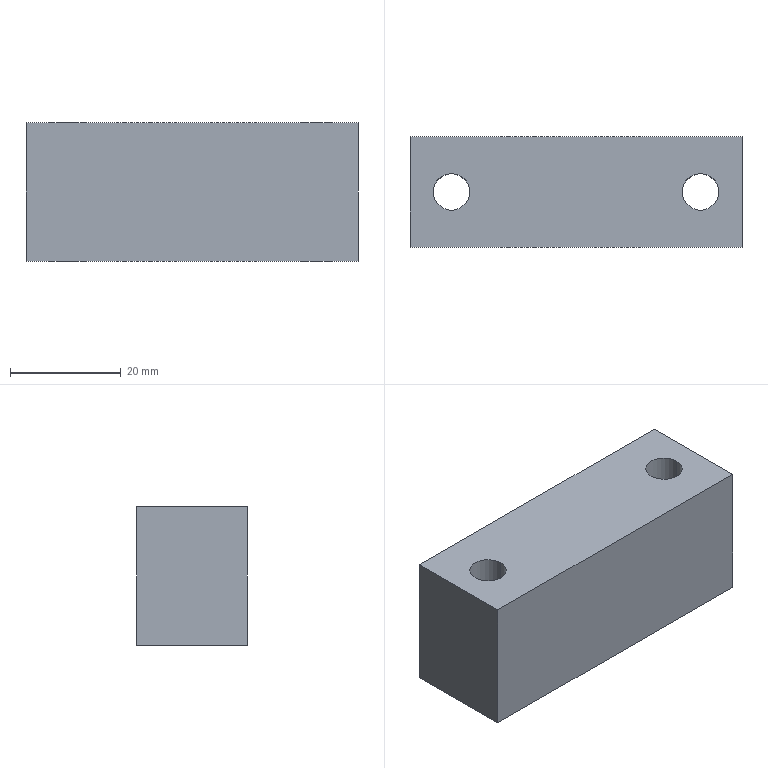Part | SolidWorks | features Extrusion 1, HoleWzd 1 | 1 solid | 10 faces | box 60 x 20 x 25 mm | volume 28289 mm3 | plane 6 | cylinder 4 | commonest cylinder face diameters 6.6 x4
STEP:
#1=CARTESIAN_POINT('',(-25.8,0.,0.));
#2=VERTEX_POINT('',#1);
#3=CARTESIAN_POINT('',(-19.2,0.,0.));
#4=VERTEX_POINT('',#3);
#5=CARTESIAN_POINT('',(-22.5,0.,0.));
#6=DIRECTION('',(0.,0.,1.));
#7=DIRECTION('',(1.,0.,0.));
#8=AXIS2_PLACEMENT_3D('',#5,#6,#7);
#9=CIRCLE('',#8,3.3);
#10=EDGE_CURVE('',#2,#4,#9,.T.);
#11=ORIENTED_EDGE('',*,*,#10,.F.);
#12=CARTESIAN_POINT('',(-25.8,0.,25.));
#13=VERTEX_POINT('',#12);
#14=CARTESIAN_POINT('',(-25.8,0.,25.));
#15=DIRECTION('',(0.,0.,1.));
#16=VECTOR('',#15,1000.);
#17=LINE('',#14,#16);
#18=EDGE_CURVE('',#2,#13,#17,.T.);
#19=ORIENTED_EDGE('',*,*,#18,.T.);
#20=CARTESIAN_POINT('',(-19.2,0.,25.));
#21=VERTEX_POINT('',#20);
#22=CARTESIAN_POINT('',(-22.5,0.,25.));
#23=DIRECTION('',(0.,0.,1.));
#24=DIRECTION('',(1.,0.,0.));
#25=AXIS2_PLACEMENT_3D('',#22,#23,#24);
#26=CIRCLE('',#25,3.3);
#27=EDGE_CURVE('',#13,#21,#26,.T.);
#28=ORIENTED_EDGE('',*,*,#27,.T.);
#29=CARTESIAN_POINT('',(-19.2,0.,25.));
#30=DIRECTION('',(0.,0.,1.));
#31=VECTOR('',#30,1000.);
#32=LINE('',#29,#31);
#33=EDGE_CURVE('',#4,#21,#32,.T.);
#34=ORIENTED_EDGE('',*,*,#33,.F.);
#35=EDGE_LOOP('',(#11,#19,#28,#34));
#36=FACE_OUTER_BOUND('',#35,.T.);
#37=CARTESIAN_POINT('',(-22.5,0.,25.));
#38=DIRECTION('',(0.,0.,1.));
#39=DIRECTION('',(1.,0.,0.));
#40=AXIS2_PLACEMENT_3D('',#37,#38,#39);
#41=CYLINDRICAL_SURFACE('',#40,3.3);
#42=ADVANCED_FACE('',(#36),#41,.F.);
#43=CARTESIAN_POINT('',(19.2,0.,0.));
#44=VERTEX_POINT('',#43);
#45=CARTESIAN_POINT('',(25.8,0.,0.));
#46=VERTEX_POINT('',#45);
#47=CARTESIAN_POINT('',(22.5,0.,0.));
#48=DIRECTION('',(0.,0.,1.));
#49=DIRECTION('',(1.,0.,0.));
#50=AXIS2_PLACEMENT_3D('',#47,#48,#49);
#51=CIRCLE('',#50,3.3);
#52=EDGE_CURVE('',#44,#46,#51,.T.);
#53=ORIENTED_EDGE('',*,*,#52,.F.);
#54=CARTESIAN_POINT('',(19.2,0.,25.));
#55=VERTEX_POINT('',#54);
#56=CARTESIAN_POINT('',(19.2,0.,25.));
#57=DIRECTION('',(0.,0.,1.));
#58=VECTOR('',#57,1000.);
#59=LINE('',#56,#58);
#60=EDGE_CURVE('',#44,#55,#59,.T.);
#61=ORIENTED_EDGE('',*,*,#60,.T.);
#62=CARTESIAN_POINT('',(25.8,0.,25.));
#63=VERTEX_POINT('',#62);
#64=CARTESIAN_POINT('',(22.5,0.,25.));
#65=DIRECTION('',(0.,0.,1.));
#66=DIRECTION('',(1.,0.,0.));
#67=AXIS2_PLACEMENT_3D('',#64,#65,#66);
#68=CIRCLE('',#67,3.3);
#69=EDGE_CURVE('',#55,#63,#68,.T.);
#70=ORIENTED_EDGE('',*,*,#69,.T.);
#71=CARTESIAN_POINT('',(25.8,0.,25.));
#72=DIRECTION('',(0.,0.,1.));
#73=VECTOR('',#72,1000.);
#74=LINE('',#71,#73);
#75=EDGE_CURVE('',#46,#63,#74,.T.);
#76=ORIENTED_EDGE('',*,*,#75,.F.);
#77=EDGE_LOOP('',(#53,#61,#70,#76));
#78=FACE_OUTER_BOUND('',#77,.T.);
#79=CARTESIAN_POINT('',(22.5,0.,25.));
#80=DIRECTION('',(0.,0.,1.));
#81=DIRECTION('',(1.,0.,0.));
#82=AXIS2_PLACEMENT_3D('',#79,#80,#81);
#83=CYLINDRICAL_SURFACE('',#82,3.3);
#84=ADVANCED_FACE('',(#78),#83,.F.);
#85=CARTESIAN_POINT('',(-30.,10.,0.));
#86=VERTEX_POINT('',#85);
#87=CARTESIAN_POINT('',(-30.,-10.,0.));
#88=VERTEX_POINT('',#87);
#89=CARTESIAN_POINT('',(-30.,-10.,0.));
#90=DIRECTION('',(0.,-1.,0.));
#91=VECTOR('',#90,1000.);
#92=LINE('',#89,#91);
#93=EDGE_CURVE('',#86,#88,#92,.T.);
#94=ORIENTED_EDGE('',*,*,#93,.T.);
#95=CARTESIAN_POINT('',(-30.,-10.,25.));
#96=VERTEX_POINT('',#95);
#97=CARTESIAN_POINT('',(-30.,-10.,25.));
#98=DIRECTION('',(0.,0.,-1.));
#99=VECTOR('',#98,1000.);
#100=LINE('',#97,#99);
#101=EDGE_CURVE('',#96,#88,#100,.T.);
#102=ORIENTED_EDGE('',*,*,#101,.F.);
#103=CARTESIAN_POINT('',(-30.,10.,25.));
#104=VERTEX_POINT('',#103);
#105=CARTESIAN_POINT('',(-30.,-10.,25.));
#106=DIRECTION('',(0.,-1.,0.));
#107=VECTOR('',#106,1000.);
#108=LINE('',#105,#107);
#109=EDGE_CURVE('',#104,#96,#108,.T.);
#110=ORIENTED_EDGE('',*,*,#109,.F.);
#111=CARTESIAN_POINT('',(-30.,10.,25.));
#112=DIRECTION('',(0.,0.,-1.));
#113=VECTOR('',#112,1000.);
#114=LINE('',#111,#113);
#115=EDGE_CURVE('',#104,#86,#114,.T.);
#116=ORIENTED_EDGE('',*,*,#115,.T.);
#117=EDGE_LOOP('',(#94,#102,#110,#116));
#118=FACE_OUTER_BOUND('',#117,.T.);
#119=CARTESIAN_POINT('',(-30.,-10.,25.));
#120=DIRECTION('',(1.,0.,0.));
#121=DIRECTION('',(0.,0.,-1.));
#122=AXIS2_PLACEMENT_3D('',#119,#120,#121);
#123=PLANE('',#122);
#124=ADVANCED_FACE('',(#118),#123,.F.);
#125=CARTESIAN_POINT('',(30.,-10.,0.));
#126=VERTEX_POINT('',#125);
#127=CARTESIAN_POINT('',(30.,-10.,0.));
#128=DIRECTION('',(1.,0.,0.));
#129=VECTOR('',#128,1000.);
#130=LINE('',#127,#129);
#131=EDGE_CURVE('',#88,#126,#130,.T.);
#132=ORIENTED_EDGE('',*,*,#131,.T.);
#133=CARTESIAN_POINT('',(30.,-10.,25.));
#134=VERTEX_POINT('',#133);
#135=CARTESIAN_POINT('',(30.,-10.,25.));
#136=DIRECTION('',(0.,0.,-1.));
#137=VECTOR('',#136,1000.);
#138=LINE('',#135,#137);
#139=EDGE_CURVE('',#134,#126,#138,.T.);
#140=ORIENTED_EDGE('',*,*,#139,.F.);
#141=CARTESIAN_POINT('',(30.,-10.,25.));
#142=DIRECTION('',(1.,0.,0.));
#143=VECTOR('',#142,1000.);
#144=LINE('',#141,#143);
#145=EDGE_CURVE('',#96,#134,#144,.T.);
#146=ORIENTED_EDGE('',*,*,#145,.F.);
#147=ORIENTED_EDGE('',*,*,#101,.T.);
#148=EDGE_LOOP('',(#132,#140,#146,#147));
#149=FACE_OUTER_BOUND('',#148,.T.);
#150=CARTESIAN_POINT('',(30.,-10.,25.));
#151=DIRECTION('',(0.,1.,0.));
#152=DIRECTION('',(-1.,0.,0.));
#153=AXIS2_PLACEMENT_3D('',#150,#151,#152);
#154=PLANE('',#153);
#155=ADVANCED_FACE('',(#149),#154,.F.);
#156=CARTESIAN_POINT('',(30.,10.,0.));
#157=VERTEX_POINT('',#156);
#158=CARTESIAN_POINT('',(30.,-10.,0.));
#159=DIRECTION('',(0.,1.,0.));
#160=VECTOR('',#159,1000.);
#161=LINE('',#158,#160);
#162=EDGE_CURVE('',#126,#157,#161,.T.);
#163=ORIENTED_EDGE('',*,*,#162,.T.);
#164=CARTESIAN_POINT('',(30.,10.,25.));
#165=VERTEX_POINT('',#164);
#166=CARTESIAN_POINT('',(30.,10.,25.));
#167=DIRECTION('',(0.,0.,-1.));
#168=VECTOR('',#167,1000.);
#169=LINE('',#166,#168);
#170=EDGE_CURVE('',#165,#157,#169,.T.);
#171=ORIENTED_EDGE('',*,*,#170,.F.);
#172=CARTESIAN_POINT('',(30.,-10.,25.));
#173=DIRECTION('',(0.,1.,0.));
#174=VECTOR('',#173,1000.);
#175=LINE('',#172,#174);
#176=EDGE_CURVE('',#134,#165,#175,.T.);
#177=ORIENTED_EDGE('',*,*,#176,.F.);
#178=ORIENTED_EDGE('',*,*,#139,.T.);
#179=EDGE_LOOP('',(#163,#171,#177,#178));
#180=FACE_OUTER_BOUND('',#179,.T.);
#181=CARTESIAN_POINT('',(30.,-10.,25.));
#182=DIRECTION('',(-1.,0.,0.));
#183=DIRECTION('',(0.,0.,1.));
#184=AXIS2_PLACEMENT_3D('',#181,#182,#183);
#185=PLANE('',#184);
#186=ADVANCED_FACE('',(#180),#185,.F.);
#187=CARTESIAN_POINT('',(30.,10.,0.));
#188=DIRECTION('',(-1.,0.,0.));
#189=VECTOR('',#188,1000.);
#190=LINE('',#187,#189);
#191=EDGE_CURVE('',#157,#86,#190,.T.);
#192=ORIENTED_EDGE('',*,*,#191,.T.);
#193=ORIENTED_EDGE('',*,*,#115,.F.);
#194=CARTESIAN_POINT('',(30.,10.,25.));
#195=DIRECTION('',(-1.,0.,0.));
#196=VECTOR('',#195,1000.);
#197=LINE('',#194,#196);
#198=EDGE_CURVE('',#165,#104,#197,.T.);
#199=ORIENTED_EDGE('',*,*,#198,.F.);
#200=ORIENTED_EDGE('',*,*,#170,.T.);
#201=EDGE_LOOP('',(#192,#193,#199,#200));
#202=FACE_OUTER_BOUND('',#201,.T.);
#203=CARTESIAN_POINT('',(30.,10.,25.));
#204=DIRECTION('',(0.,-1.,0.));
#205=DIRECTION('',(1.,0.,0.));
#206=AXIS2_PLACEMENT_3D('',#203,#204,#205);
#207=PLANE('',#206);
#208=ADVANCED_FACE('',(#202),#207,.F.);
#209=CARTESIAN_POINT('',(-22.5,0.,25.));
#210=DIRECTION('',(0.,0.,1.));
#211=DIRECTION('',(1.,0.,0.));
#212=AXIS2_PLACEMENT_3D('',#209,#210,#211);
#213=CIRCLE('',#212,3.3);
#214=EDGE_CURVE('',#21,#13,#213,.T.);
#215=ORIENTED_EDGE('',*,*,#214,.F.);
#216=ORIENTED_EDGE('',*,*,#27,.F.);
#217=EDGE_LOOP('',(#215,#216));
#218=FACE_BOUND('',#217,.T.);
#219=CARTESIAN_POINT('',(22.5,0.,25.));
#220=DIRECTION('',(0.,0.,1.));
#221=DIRECTION('',(1.,0.,0.));
#222=AXIS2_PLACEMENT_3D('',#219,#220,#221);
#223=CIRCLE('',#222,3.3);
#224=EDGE_CURVE('',#63,#55,#223,.T.);
#225=ORIENTED_EDGE('',*,*,#224,.F.);
#226=ORIENTED_EDGE('',*,*,#69,.F.);
#227=EDGE_LOOP('',(#225,#226));
#228=FACE_BOUND('',#227,.T.);
#229=ORIENTED_EDGE('',*,*,#109,.T.);
#230=ORIENTED_EDGE('',*,*,#145,.T.);
#231=ORIENTED_EDGE('',*,*,#176,.T.);
#232=ORIENTED_EDGE('',*,*,#198,.T.);
#233=EDGE_LOOP('',(#229,#230,#231,#232));
#234=FACE_OUTER_BOUND('',#233,.T.);
#235=CARTESIAN_POINT('',(0.,0.,25.));
#236=DIRECTION('',(0.,0.,1.));
#237=DIRECTION('',(1.,0.,0.));
#238=AXIS2_PLACEMENT_3D('',#235,#236,#237);
#239=PLANE('',#238);
#240=ADVANCED_FACE('',(#218,#228,#234),#239,.T.);
#241=CARTESIAN_POINT('',(-22.5,0.,0.));
#242=DIRECTION('',(0.,0.,1.));
#243=DIRECTION('',(1.,0.,0.));
#244=AXIS2_PLACEMENT_3D('',#241,#242,#243);
#245=CIRCLE('',#244,3.3);
#246=EDGE_CURVE('',#4,#2,#245,.T.);
#247=ORIENTED_EDGE('',*,*,#246,.T.);
#248=ORIENTED_EDGE('',*,*,#10,.T.);
#249=EDGE_LOOP('',(#247,#248));
#250=FACE_BOUND('',#249,.T.);
#251=CARTESIAN_POINT('',(22.5,0.,0.));
#252=DIRECTION('',(0.,0.,1.));
#253=DIRECTION('',(1.,0.,0.));
#254=AXIS2_PLACEMENT_3D('',#251,#252,#253);
#255=CIRCLE('',#254,3.3);
#256=EDGE_CURVE('',#46,#44,#255,.T.);
#257=ORIENTED_EDGE('',*,*,#256,.T.);
#258=ORIENTED_EDGE('',*,*,#52,.T.);
#259=EDGE_LOOP('',(#257,#258));
#260=FACE_BOUND('',#259,.T.);
#261=ORIENTED_EDGE('',*,*,#93,.F.);
#262=ORIENTED_EDGE('',*,*,#191,.F.);
#263=ORIENTED_EDGE('',*,*,#162,.F.);
#264=ORIENTED_EDGE('',*,*,#131,.F.);
#265=EDGE_LOOP('',(#261,#262,#263,#264));
#266=FACE_OUTER_BOUND('',#265,.T.);
#267=CARTESIAN_POINT('',(0.,0.,0.));
#268=DIRECTION('',(0.,0.,1.));
#269=DIRECTION('',(1.,0.,0.));
#270=AXIS2_PLACEMENT_3D('',#267,#268,#269);
#271=PLANE('',#270);
#272=ADVANCED_FACE('',(#250,#260,#266),#271,.F.);
#273=ORIENTED_EDGE('',*,*,#60,.F.);
#274=ORIENTED_EDGE('',*,*,#256,.F.);
#275=ORIENTED_EDGE('',*,*,#75,.T.);
#276=ORIENTED_EDGE('',*,*,#224,.T.);
#277=EDGE_LOOP('',(#273,#274,#275,#276));
#278=FACE_OUTER_BOUND('',#277,.T.);
#279=CARTESIAN_POINT('',(22.5,0.,25.));
#280=DIRECTION('',(0.,0.,1.));
#281=DIRECTION('',(1.,0.,0.));
#282=AXIS2_PLACEMENT_3D('',#279,#280,#281);
#283=CYLINDRICAL_SURFACE('',#282,3.3);
#284=ADVANCED_FACE('',(#278),#283,.F.);
#285=ORIENTED_EDGE('',*,*,#18,.F.);
#286=ORIENTED_EDGE('',*,*,#246,.F.);
#287=ORIENTED_EDGE('',*,*,#33,.T.);
#288=ORIENTED_EDGE('',*,*,#214,.T.);
#289=EDGE_LOOP('',(#285,#286,#287,#288));
#290=FACE_OUTER_BOUND('',#289,.T.);
#291=CARTESIAN_POINT('',(-22.5,0.,25.));
#292=DIRECTION('',(0.,0.,1.));
#293=DIRECTION('',(1.,0.,0.));
#294=AXIS2_PLACEMENT_3D('',#291,#292,#293);
#295=CYLINDRICAL_SURFACE('',#294,3.3);
#296=ADVANCED_FACE('',(#290),#295,.F.);
#297=CLOSED_SHELL('',(#42,#84,#124,#155,#186,#208,#240,#272,#284,#296));
#298=MANIFOLD_SOLID_BREP('',#297);
#299=CARTESIAN_POINT('',(0.,0.,0.));
#300=DIRECTION('',(0.,0.,1.));
#301=DIRECTION('',(1.,0.,0.));
#302=AXIS2_PLACEMENT_3D('',#299,#300,#301);
#303=(LENGTH_UNIT()NAMED_UNIT(*)SI_UNIT(.MILLI.,.METRE.));
#304=UNCERTAINTY_MEASURE_WITH_UNIT(LENGTH_MEASURE(0.00001),#303,'','');
#305=(NAMED_UNIT(*)PLANE_ANGLE_UNIT()SI_UNIT($,.RADIAN.));
#306=(NAMED_UNIT(*)SI_UNIT($,.STERADIAN.)SOLID_ANGLE_UNIT());
#307=(GEOMETRIC_REPRESENTATION_CONTEXT(3)GLOBAL_UNCERTAINTY_ASSIGNED_CONTEXT((#304))GLOBAL_UNIT_ASSIGNED_CONTEXT((#303,#305,#306))REPRESENTATION_CONTEXT('',''));
#308=ADVANCED_BREP_SHAPE_REPRESENTATION('',(#298,#302),#307);